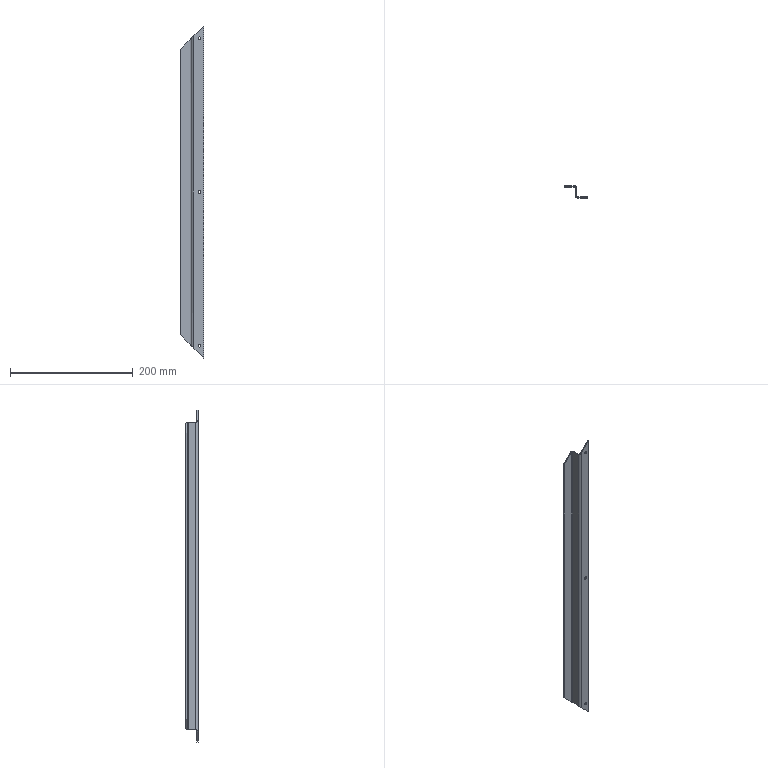Part | STEP file | SYL_0392D6J1SYL0380DJ100-543650 | 1 solid | 28 faces | box 38 x 20 x 540 mm | volume 53472 mm3 | plane 14 | cylinder 10 | spline 4 | commonest cylinder face diameters 4.5 x6 4 x2 8 x2